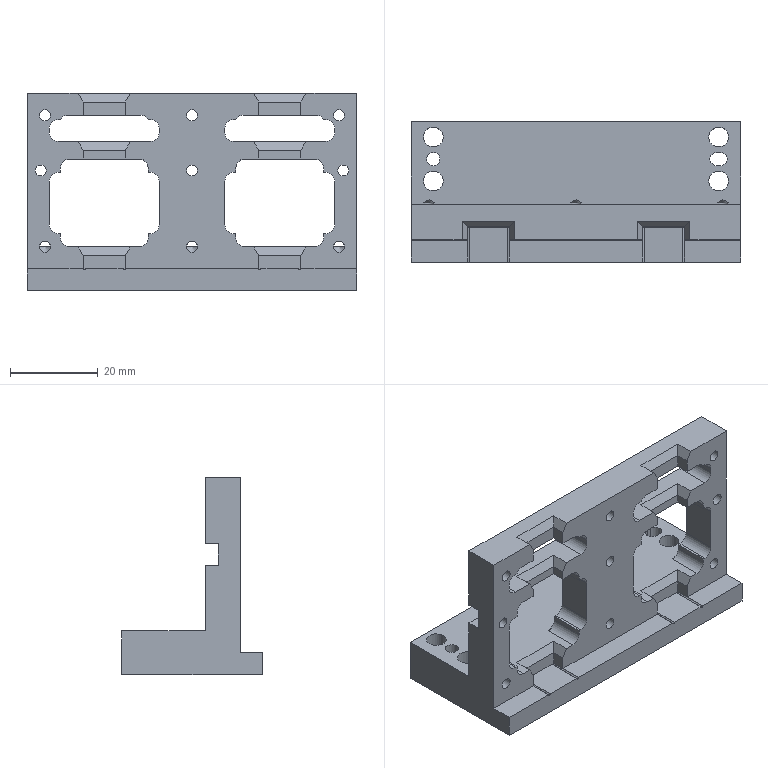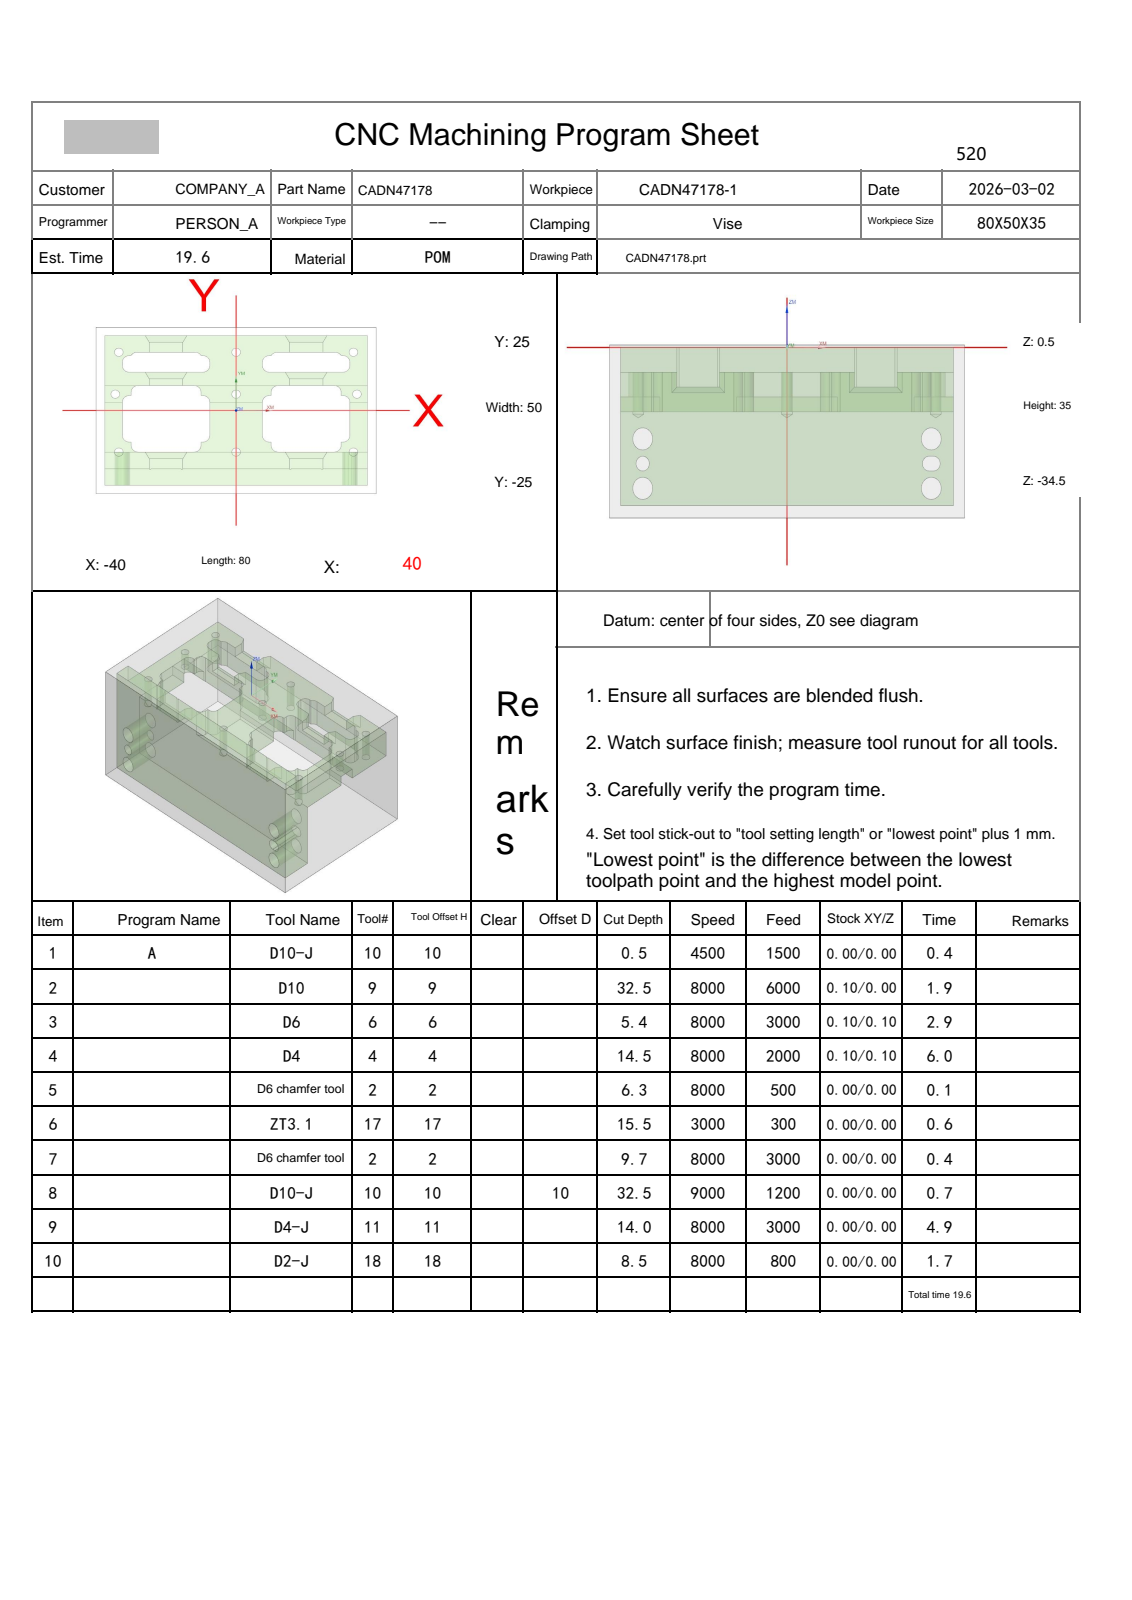NC program | NX | posted by the shop | part box 75 x 32 x 45 mm
Lines 1 to 1488 of 18359:
%
O0001
(Machine time: 21.50 MIN)
(===Total Tool:8===)
(T10=D10-J  D=10.  R=0.   D-  H10 Z=-32.  )
(T9=D10     D=10.  R=0.   D-  H09 Z=-32.  )
(T6=D6      D=6.   R=0.   D-  H06 Z=-4.9  )
(T4=D4      D=4.   R=0.   D-  H04 Z=-14.  )
(T2=D6 chamfer tool   D=6.   R=0.   D-  H02 Z=-9.2  )
(T17=ZT3.1  D=3.1  DR_a=118 D-  H17 Z=-15.  )
(T11=D4-J   D=4.   R=0.   D11 H11 Z=-13.52)
(T18=D2-J   D=2.   R=0.   D-  H18 Z=-8.   )
G80 G90 G17 G49 G40
G91 G28 Z0
M01
N1 T10 M06
(D10-J  D=10. R=0. H=10 ce=0.00 di=0.00)
G00 G90 G54 X47.5 Y-20.625 M03 S4500
G43 H10 Z30.
M08
Z2.
G01 Z0.0 F1500.
X42.5
X-42.5
Y-13.75
X42.5
Y-6.875
X-42.5
Y0.0
X42.5
Y6.875
X-42.5
Y13.75
X42.5
Y20.625
X-42.5
X-47.5
Z2.
G00 Z30.
G91 G28 Z0.0
M05
M09
G91 G28 Z0.0
M01
N2 T09 M06
(D10  D=10. R=0. H=09 ce=0.10 di=0.00)
G00 G90 G54 X0.0 Y-27.6 M03 S8000
G43 H09 Z30.
M08
Z.5
G01 X-37.5 Z.391 F6000.
G02 X-42.6 Y-22.5 Z.367 I0.0 J5.1
G01 Y22.5 Z.236
G02 X-37.5 Y27.6 Z.213 I5.1 J0.0
G01 X37.5 Z-.006
G02 X42.6 Y22.5 Z-.029 I0.0 J-5.1
G01 Y-22.5 Z-.16
G02 X37.5 Y-27.6 Z-.183 I-5.1 J0.0
G01 X-37.5 Z-.402
G02 X-42.6 Y-22.5 Z-.425 I0.0 J5.1
G01 Y22.5 Z-.556
G02 X-37.5 Y27.6 Z-.58 I5.1 J0.0
G01 X37.5 Z-.798
G02 X42.6 Y22.5 Z-.822 I0.0 J-5.1
G01 Y-22.5 Z-.953
G02 X37.5 Y-27.6 Z-.976 I-5.1 J0.0
G01 X-37.5 Z-1.195
G02 X-42.6 Y-22.5 Z-1.218 I0.0 J5.1
G01 Y22.5 Z-1.349
G02 X-37.5 Y27.6 Z-1.372 I5.1 J0.0
G01 X37.5 Z-1.591
G02 X42.6 Y22.5 Z-1.614 I0.0 J-5.1
G01 Y-22.5 Z-1.745
G02 X37.5 Y-27.6 Z-1.769 I-5.1 J0.0
G01 X-37.5 Z-1.987
G02 X-42.6 Y-22.5 Z-2.011 I0.0 J5.1
G01 Y22.5 Z-2.142
G02 X-37.5 Y27.6 Z-2.165 I5.1 J0.0
G01 X37.5 Z-2.384
G02 X42.6 Y22.5 Z-2.407 I0.0 J-5.1
G01 Y-22.5 Z-2.538
G02 X37.5 Y-27.6 Z-2.561 I-5.1 J0.0
G01 X-37.5 Z-2.78
G02 X-42.6 Y-22.5 Z-2.803 I0.0 J5.1
G01 Y22.5 Z-2.934
G02 X-37.5 Y27.6 Z-2.958 I5.1 J0.0
G01 X37.5 Z-3.176
G02 X42.6 Y22.5 Z-3.2 I0.0 J-5.1
G01 Y-22.5 Z-3.331
G02 X37.5 Y-27.6 Z-3.354 I-5.1 J0.0
G01 X-37.5 Z-3.573
G02 X-42.6 Y-22.5 Z-3.596 I0.0 J5.1
G01 Y22.5 Z-3.727
G02 X-37.5 Y27.6 Z-3.75 I5.1 J0.0
G01 X37.5 Z-3.969
G02 X42.6 Y22.5 Z-3.992 I0.0 J-5.1
G01 Y-22.5 Z-4.123
G02 X37.5 Y-27.6 Z-4.147 I-5.1 J0.0
G01 X-37.5 Z-4.365
G02 X-42.6 Y-22.5 Z-4.389 I0.0 J5.1
G01 Y22.5 Z-4.52
G02 X-37.5 Y27.6 Z-4.543 I5.1 J0.0
G01 X37.5 Z-4.762
G02 X42.6 Y22.5 Z-4.785 I0.0 J-5.1
G01 Y-22.5 Z-4.916
G02 X37.5 Y-27.6 Z-4.94 I-5.1 J0.0
G01 X-37.5 Z-5.158
G02 X-42.6 Y-22.5 Z-5.181 I0.0 J5.1
G01 Y22.5 Z-5.313
G02 X-37.5 Y27.6 Z-5.336 I5.1 J0.0
G01 X37.5 Z-5.554
G02 X42.6 Y22.5 Z-5.578 I0.0 J-5.1
G01 Y-22.5 Z-5.709
G02 X37.5 Y-27.6 Z-5.732 I-5.1 J0.0
G01 X-37.5 Z-5.951
G02 X-42.6 Y-22.5 Z-5.974 I0.0 J5.1
G01 Y22.5 Z-6.105
G02 X-37.5 Y27.6 Z-6.129 I5.1 J0.0
G01 X37.5 Z-6.347
G02 X42.6 Y22.5 Z-6.37 I0.0 J-5.1
G01 Y-22.5 Z-6.502
G02 X37.5 Y-27.6 Z-6.525 I-5.1 J0.0
G01 X-37.5 Z-6.743
G02 X-42.6 Y-22.5 Z-6.767 I0.0 J5.1
G01 Y22.5 Z-6.898
G02 X-37.5 Y27.6 Z-6.921 I5.1 J0.0
G01 X37.5 Z-7.14
G02 X42.6 Y22.5 Z-7.163 I0.0 J-5.1
G01 Y-22.5 Z-7.294
G02 X37.5 Y-27.6 Z-7.318 I-5.1 J0.0
G01 X-37.5 Z-7.536
G02 X-42.6 Y-22.5 Z-7.559 I0.0 J5.1
G01 Y22.5 Z-7.691
G02 X-37.5 Y27.6 Z-7.714 I5.1 J0.0
G01 X37.5 Z-7.932
G02 X42.6 Y22.5 Z-7.956 I0.0 J-5.1
G01 Y-22.5 Z-8.087
G02 X37.5 Y-27.6 Z-8.11 I-5.1 J0.0
G01 X-37.5 Z-8.329
G02 X-42.6 Y-22.5 Z-8.352 I0.0 J5.1
G01 Y22.5 Z-8.483
G02 X-37.5 Y27.6 Z-8.507 I5.1 J0.0
G01 X37.5 Z-8.725
G02 X42.6 Y22.5 Z-8.748 I0.0 J-5.1
G01 Y-22.5 Z-8.88
G02 X37.5 Y-27.6 Z-8.903 I-5.1 J0.0
G01 X-37.5 Z-9.121
G02 X-42.6 Y-22.5 Z-9.145 I0.0 J5.1
G01 Y22.5 Z-9.276
G02 X-37.5 Y27.6 Z-9.299 I5.1 J0.0
G01 X37.5 Z-9.518
G02 X42.6 Y22.5 Z-9.541 I0.0 J-5.1
G01 Y-22.5 Z-9.672
G02 X37.5 Y-27.6 Z-9.696 I-5.1 J0.0
G01 X-37.5 Z-9.914
G02 X-42.6 Y-22.5 Z-9.937 I0.0 J5.1
G01 Y22.5 Z-10.069
G02 X-37.5 Y27.6 Z-10.092 I5.1 J0.0
G01 X37.5 Z-10.31
G02 X42.6 Y22.5 Z-10.334 I0.0 J-5.1
G01 Y-22.5 Z-10.465
G02 X37.5 Y-27.6 Z-10.488 I-5.1 J0.0
G01 X-37.5 Z-10.707
G02 X-42.6 Y-22.5 Z-10.73 I0.0 J5.1
G01 Y22.5 Z-10.861
G02 X-37.5 Y27.6 Z-10.885 I5.1 J0.0
G01 X37.5 Z-11.103
G02 X42.6 Y22.5 Z-11.127 I0.0 J-5.1
G01 Y-22.5 Z-11.258
G02 X37.5 Y-27.6 Z-11.281 I-5.1 J0.0
G01 X-37.5 Z-11.5
G02 X-42.6 Y-22.5 Z-11.523 I0.0 J5.1
G01 Y22.5 Z-11.654
G02 X-37.5 Y27.6 Z-11.677 I5.1 J0.0
G01 X37.5 Z-11.896
G02 X42.6 Y22.5 Z-11.919 I0.0 J-5.1
G01 Y-22.5 Z-12.05
G02 X37.5 Y-27.6 Z-12.074 I-5.1 J0.0
G01 X-37.5 Z-12.292
G02 X-42.6 Y-22.5 Z-12.316 I0.0 J5.1
G01 Y22.5 Z-12.447
G02 X-37.5 Y27.6 Z-12.47 I5.1 J0.0
G01 X37.5 Z-12.689
G02 X42.6 Y22.5 Z-12.712 I0.0 J-5.1
G01 Y-22.5 Z-12.843
G02 X37.5 Y-27.6 Z-12.866 I-5.1 J0.0
G01 X-37.5 Z-13.085
G02 X-42.6 Y-22.5 Z-13.108 I0.0 J5.1
G01 Y22.5 Z-13.239
G02 X-37.5 Y27.6 Z-13.263 I5.1 J0.0
G01 X37.5 Z-13.481
G02 X42.6 Y22.5 Z-13.505 I0.0 J-5.1
G01 Y-22.5 Z-13.636
G02 X37.5 Y-27.6 Z-13.659 I-5.1 J0.0
G01 X-37.5 Z-13.878
G02 X-42.6 Y-22.5 Z-13.901 I0.0 J5.1
G01 Y22.5 Z-14.032
G02 X-37.5 Y27.6 Z-14.055 I5.1 J0.0
G01 X37.5 Z-14.274
G02 X42.6 Y22.5 Z-14.297 I0.0 J-5.1
G01 Y-22.5 Z-14.428
G02 X37.5 Y-27.6 Z-14.452 I-5.1 J0.0
G01 X-37.5 Z-14.67
G02 X-42.6 Y-22.5 Z-14.694 I0.0 J5.1
G01 Y22.5 Z-14.825
G02 X-37.5 Y27.6 Z-14.848 I5.1 J0.0
G01 X37.5 Z-15.067
G02 X42.6 Y22.5 Z-15.09 I0.0 J-5.1
G01 Y-22.5 Z-15.221
G02 X37.5 Y-27.6 Z-15.244 I-5.1 J0.0
G01 X-37.5 Z-15.463
G02 X-42.6 Y-22.5 Z-15.486 I0.0 J5.1
G01 Y22.5 Z-15.617
G02 X-37.5 Y27.6 Z-15.641 I5.1 J0.0
G01 X37.5 Z-15.859
G02 X42.6 Y22.5 Z-15.883 I0.0 J-5.1
G01 Y-22.5 Z-16.014
G02 X37.5 Y-27.6 Z-16.037 I-5.1 J0.0
G01 X-37.5 Z-16.256
G02 X-42.6 Y-22.5 Z-16.279 I0.0 J5.1
G01 Y22.5 Z-16.41
G02 X-37.5 Y27.6 Z-16.433 I5.1 J0.0
G01 X37.5 Z-16.652
G02 X42.6 Y22.5 Z-16.675 I0.0 J-5.1
G01 Y-22.5 Z-16.806
G02 X37.5 Y-27.6 Z-16.83 I-5.1 J0.0
G01 X-37.5 Z-17.048
G02 X-42.6 Y-22.5 Z-17.072 I0.0 J5.1
G01 Y22.5 Z-17.203
G02 X-37.5 Y27.6 Z-17.226 I5.1 J0.0
G01 X37.5 Z-17.445
G02 X42.6 Y22.5 Z-17.468 I0.0 J-5.1
G01 Y-22.5 Z-17.599
G02 X37.5 Y-27.6 Z-17.622 I-5.1 J0.0
G01 X-37.5 Z-17.841
G02 X-42.6 Y-22.5 Z-17.864 I0.0 J5.1
G01 Y22.5 Z-17.995
G02 X-37.5 Y27.6 Z-18.019 I5.1 J0.0
G01 X37.5 Z-18.237
G02 X42.6 Y22.5 Z-18.261 I0.0 J-5.1
G01 Y-22.5 Z-18.392
G02 X37.5 Y-27.6 Z-18.415 I-5.1 J0.0
G01 X-37.5 Z-18.634
G02 X-42.6 Y-22.5 Z-18.657 I0.0 J5.1
G01 Y22.5 Z-18.788
G02 X-37.5 Y27.6 Z-18.811 I5.1 J0.0
G01 X37.5 Z-19.03
G02 X42.6 Y22.5 Z-19.053 I0.0 J-5.1
G01 Y-22.5 Z-19.184
G02 X37.5 Y-27.6 Z-19.208 I-5.1 J0.0
G01 X-37.5 Z-19.426
G02 X-42.6 Y-22.5 Z-19.45 I0.0 J5.1
G01 Y22.5 Z-19.581
G02 X-37.5 Y27.6 Z-19.604 I5.1 J0.0
G01 X37.5 Z-19.823
G02 X42.6 Y22.5 Z-19.846 I0.0 J-5.1
G01 Y-22.5 Z-19.977
G02 X37.5 Y-27.6 Z-20. I-5.1 J0.0
G01 X-37.5 Z-20.219
G02 X-42.6 Y-22.5 Z-20.242 I0.0 J5.1
G01 Y22.5 Z-20.373
G02 X-37.5 Y27.6 Z-20.397 I5.1 J0.0
G01 X37.5 Z-20.615
G02 X42.6 Y22.5 Z-20.639 I0.0 J-5.1
G01 Y-22.5 Z-20.77
G02 X37.5 Y-27.6 Z-20.793 I-5.1 J0.0
G01 X-37.5 Z-21.012
G02 X-42.6 Y-22.5 Z-21.035 I0.0 J5.1
G01 Y22.5 Z-21.166
G02 X-37.5 Y27.6 Z-21.19 I5.1 J0.0
G01 X37.5 Z-21.408
G02 X42.6 Y22.5 Z-21.431 I0.0 J-5.1
G01 Y-22.5 Z-21.563
G02 X37.5 Y-27.6 Z-21.586 I-5.1 J0.0
G01 X-37.5 Z-21.804
G02 X-42.6 Y-22.5 Z-21.828 I0.0 J5.1
G01 Y22.5 Z-21.959
G02 X-37.5 Y27.6 Z-21.982 I5.1 J0.0
G01 X37.5 Z-22.201
G02 X42.6 Y22.5 Z-22.224 I0.0 J-5.1
G01 Y-22.5 Z-22.355
G02 X37.5 Y-27.6 Z-22.379 I-5.1 J0.0
G01 X-37.5 Z-22.597
G02 X-42.6 Y-22.5 Z-22.62 I0.0 J5.1
G01 Y22.5 Z-22.752
G02 X-37.5 Y27.6 Z-22.775 I5.1 J0.0
G01 X37.5 Z-22.993
G02 X42.6 Y22.5 Z-23.017 I0.0 J-5.1
G01 Y-22.5 Z-23.148
G02 X37.5 Y-27.6 Z-23.171 I-5.1 J0.0
G01 X-37.5 Z-23.39
G02 X-42.6 Y-22.5 Z-23.413 I0.0 J5.1
G01 Y22.5 Z-23.544
G02 X-37.5 Y27.6 Z-23.568 I5.1 J0.0
G01 X37.5 Z-23.786
G02 X42.6 Y22.5 Z-23.809 I0.0 J-5.1
G01 Y-22.5 Z-23.941
G02 X37.5 Y-27.6 Z-23.964 I-5.1 J0.0
G01 X-37.5 Z-24.182
G02 X-42.6 Y-22.5 Z-24.206 I0.0 J5.1
G01 Y22.5 Z-24.337
G02 X-37.5 Y27.6 Z-24.36 I5.1 J0.0
G01 X37.5 Z-24.579
G02 X42.6 Y22.5 Z-24.602 I0.0 J-5.1
G01 Y-22.5 Z-24.733
G02 X37.5 Y-27.6 Z-24.757 I-5.1 J0.0
G01 X-37.5 Z-24.975
G02 X-42.6 Y-22.5 Z-24.998 I0.0 J5.1
G01 Y22.5 Z-25.13
G02 X-37.5 Y27.6 Z-25.153 I5.1 J0.0
G01 X37.5 Z-25.371
G02 X42.6 Y22.5 Z-25.395 I0.0 J-5.1
G01 Y-22.5 Z-25.526
G02 X37.5 Y-27.6 Z-25.549 I-5.1 J0.0
G01 X-37.5 Z-25.768
G02 X-42.6 Y-22.5 Z-25.791 I0.0 J5.1
G01 Y22.5 Z-25.922
G02 X-37.5 Y27.6 Z-25.946 I5.1 J0.0
G01 X37.5 Z-26.164
G02 X42.6 Y22.5 Z-26.187 I0.0 J-5.1
G01 Y-22.5 Z-26.319
G02 X37.5 Y-27.6 Z-26.342 I-5.1 J0.0
G01 X-37.5 Z-26.56
G02 X-42.6 Y-22.5 Z-26.584 I0.0 J5.1
G01 Y22.5 Z-26.715
G02 X-37.5 Y27.6 Z-26.738 I5.1 J0.0
G01 X37.5 Z-26.957
G02 X42.6 Y22.5 Z-26.98 I0.0 J-5.1
G01 Y-22.5 Z-27.111
G02 X37.5 Y-27.6 Z-27.135 I-5.1 J0.0
G01 X-37.5 Z-27.353
G02 X-42.6 Y-22.5 Z-27.377 I0.0 J5.1
G01 Y22.5 Z-27.508
G02 X-37.5 Y27.6 Z-27.531 I5.1 J0.0
G01 X37.5 Z-27.75
G02 X42.6 Y22.5 Z-27.773 I0.0 J-5.1
G01 Y-22.5 Z-27.904
G02 X37.5 Y-27.6 Z-27.927 I-5.1 J0.0
G01 X-37.5 Z-28.146
G02 X-42.6 Y-22.5 Z-28.169 I0.0 J5.1
G01 Y22.5 Z-28.3
G02 X-37.5 Y27.6 Z-28.324 I5.1 J0.0
G01 X37.5 Z-28.542
G02 X42.6 Y22.5 Z-28.566 I0.0 J-5.1
G01 Y-22.5 Z-28.697
G02 X37.5 Y-27.6 Z-28.72 I-5.1 J0.0
G01 X-37.5 Z-28.939
G02 X-42.6 Y-22.5 Z-28.962 I0.0 J5.1
G01 Y22.5 Z-29.093
G02 X-37.5 Y27.6 Z-29.116 I5.1 J0.0
G01 X37.5 Z-29.335
G02 X42.6 Y22.5 Z-29.358 I0.0 J-5.1
G01 Y-22.5 Z-29.489
G02 X37.5 Y-27.6 Z-29.513 I-5.1 J0.0
G01 X-37.5 Z-29.731
G02 X-42.6 Y-22.5 Z-29.755 I0.0 J5.1
G01 Y22.5 Z-29.886
G02 X-37.5 Y27.6 Z-29.909 I5.1 J0.0
G01 X37.5 Z-30.128
G02 X42.6 Y22.5 Z-30.151 I0.0 J-5.1
G01 Y-22.5 Z-30.282
G02 X37.5 Y-27.6 Z-30.305 I-5.1 J0.0
G01 X-37.5 Z-30.524
G02 X-42.6 Y-22.5 Z-30.547 I0.0 J5.1
G01 Y22.5 Z-30.678
G02 X-37.5 Y27.6 Z-30.702 I5.1 J0.0
G01 X37.5 Z-30.92
G02 X42.6 Y22.5 Z-30.944 I0.0 J-5.1
G01 Y-22.5 Z-31.075
G02 X37.5 Y-27.6 Z-31.098 I-5.1 J0.0
G01 X-37.5 Z-31.317
G02 X-42.6 Y-22.5 Z-31.34 I0.0 J5.1
G01 Y22.5 Z-31.471
G02 X-37.5 Y27.6 Z-31.494 I5.1 J0.0
G01 X37.5 Z-31.713
G02 X42.6 Y22.5 Z-31.736 I0.0 J-5.1
G01 Y-22.5 Z-31.867
G02 X37.5 Y-27.6 Z-31.891 I-5.1 J0.0
G01 X0.0 Z-32.
X-37.5
G02 X-42.6 Y-22.5 I0.0 J5.1
G01 Y22.5
G02 X-37.5 Y27.6 I5.1 J0.0
G01 X37.5
G02 X42.6 Y22.5 I0.0 J-5.1
G01 Y-22.5
G02 X37.5 Y-27.6 I-5.1 J0.0
G01 X0.0
X-.5
Z-31.
G00 Z30.
G91 G28 Z0.0
M05
M09
G91 G28 Z0.0
M01
N3 T06 M06
(D6  D=6. R=0. H=06 ce=0.10 di=0.10)
G00 G90 G54 X0.0 Y28.5 M03 S8000
G43 H06 Z10.5
M08
Z1.01
G01 Z-.49 F3000.
Y25.44
X40.44
Y-14.4
X24.8
G03 X24.55 Y-14.41 I0.0 J-3.1
X24.3 Y-14.4 I-.25 J-3.09
G01 X15.7
G03 X15.45 Y-14.41 I0.0 J-3.1
X15.2 Y-14.4 I-.25 J-3.09
G01 X-15.2
G03 X-15.45 Y-14.41 I0.0 J-3.1
X-15.7 Y-14.4 I-.25 J-3.09
G01 X-24.3
G03 X-24.55 Y-14.41 I0.0 J-3.1
X-24.8 Y-14.4 I-.25 J-3.09
G01 X-40.44
Y25.44
X-1.821
G02 X-1.322 Y25.173 I0.0 J-.6
G01 X1.322 Y21.207
G03 X1.821 Y20.94 I.499 J.333
G01 X35.342
G02 X35.94 Y20.342 I-.002 J-.6
G01 Y-9.302
G02 X35.342 Y-9.9 I-.6 J.002
G01 X24.8
G03 X24.55 Y-9.904 I0.0 J-7.6
X24.3 Y-9.9 I-.25 J-7.596
G01 X15.7
G03 X15.45 Y-9.904 I0.0 J-7.6
X15.2 Y-9.9 I-.25 J-7.596
G01 X-15.2
G03 X-15.45 Y-9.904 I0.0 J-7.6
X-15.7 Y-9.9 I-.25 J-7.596
G01 X-24.3
G03 X-24.55 Y-9.904 I0.0 J-7.6
X-24.8 Y-9.9 I-.25 J-7.596
G01 X-35.342
G02 X-35.94 Y-9.302 I.002 J.6
G01 Y20.342
G02 X-35.342 Y20.94 I.6 J-.002
G01 X-1.821
G02 X-1.322 Y20.673 I0.0 J-.6
G01 X1.322 Y16.707
G03 X1.821 Y16.44 I.499 J.333
G01 X30.842
G02 X31.44 Y15.842 I-.002 J-.6
G01 Y-4.802
G02 X30.842 Y-5.4 I-.6 J.002
G01 X24.8
G03 X24.55 Y-5.403 I0.0 J-12.1
X24.3 Y-5.4 I-.25 J-12.097
G01 X15.7
G03 X15.45 Y-5.403 I0.0 J-12.1
X15.2 Y-5.4 I-.25 J-12.097
G01 X-15.2
G03 X-15.45 Y-5.403 I0.0 J-12.1
X-15.7 Y-5.4 I-.25 J-12.097
G01 X-24.3
G03 X-24.55 Y-5.403 I0.0 J-12.1
X-24.8 Y-5.4 I-.25 J-12.097
G01 X-30.842
G02 X-31.44 Y-4.802 I.002 J.6
G01 Y15.842
G02 X-30.842 Y16.44 I.6 J-.002
G01 X-1.821
G02 X-1.322 Y16.173 I0.0 J-.6
G01 X1.322 Y12.207
G03 X1.821 Y11.94 I.499 J.333
G01 X26.342
G02 X26.94 Y11.342 I-.002 J-.6
G01 Y-.302
G02 X26.342 Y-.9 I-.6 J.002
G01 X24.8
G03 X24.55 Y-.902 I0.0 J-16.6
X24.3 Y-.9 I-.25 J-16.598
G01 X15.7
G03 X15.45 Y-.902 I0.0 J-16.6
X15.2 Y-.9 I-.25 J-16.598
G01 X-15.2
G03 X-15.45 Y-.902 I0.0 J-16.6
X-15.7 Y-.9 I-.25 J-16.598
G01 X-24.3
G03 X-24.55 Y-.902 I0.0 J-16.6
X-24.8 Y-.9 I-.25 J-16.598
G01 X-26.342
G02 X-26.94 Y-.302 I.002 J.6
G01 Y11.342
G02 X-26.342 Y11.94 I.6 J-.002
G01 X-1.821
G02 X-1.322 Y11.673 I0.0 J-.6
G01 X1.322 Y7.707
G03 X1.821 Y7.44 I.499 J.333
G01 X21.842
G02 X22.44 Y6.842 I-.002 J-.6
G01 Y4.198
G02 X21.842 Y3.6 I-.6 J.002
G01 X-21.842
G02 X-22.44 Y4.198 I.002 J.6
G01 Y6.842
G02 X-21.842 Y7.44 I.6 J-.002
G01 X0.0
X.5
Y10.44
Z1.01
G00 X0.0 Y28.5
Z.52
G01 Z-.98
Y25.44
X40.44
Y-14.4
X24.8
G03 X24.55 Y-14.41 I0.0 J-3.1
X24.3 Y-14.4 I-.25 J-3.09
G01 X15.7
G03 X15.45 Y-14.41 I0.0 J-3.1
X15.2 Y-14.4 I-.25 J-3.09
G01 X-15.2
G03 X-15.45 Y-14.41 I0.0 J-3.1
X-15.7 Y-14.4 I-.25 J-3.09
G01 X-24.3
G03 X-24.55 Y-14.41 I0.0 J-3.1
X-24.8 Y-14.4 I-.25 J-3.09
G01 X-40.44
Y25.44
X-1.821
G02 X-1.322 Y25.173 I0.0 J-.6
G01 X1.322 Y21.207
G03 X1.821 Y20.94 I.499 J.333
G01 X35.342
G02 X35.94 Y20.342 I-.002 J-.6
G01 Y-9.302
G02 X35.342 Y-9.9 I-.6 J.002
G01 X24.8
G03 X24.55 Y-9.904 I0.0 J-7.6
X24.3 Y-9.9 I-.25 J-7.596
G01 X15.7
G03 X15.45 Y-9.904 I0.0 J-7.6
X15.2 Y-9.9 I-.25 J-7.596
G01 X-15.2
G03 X-15.45 Y-9.904 I0.0 J-7.6
X-15.7 Y-9.9 I-.25 J-7.596
G01 X-24.3
G03 X-24.55 Y-9.904 I0.0 J-7.6
X-24.8 Y-9.9 I-.25 J-7.596
G01 X-35.342
G02 X-35.94 Y-9.302 I.002 J.6
G01 Y20.342
G02 X-35.342 Y20.94 I.6 J-.002
G01 X-1.821
G02 X-1.322 Y20.673 I0.0 J-.6
G01 X1.322 Y16.707
G03 X1.821 Y16.44 I.499 J.333
G01 X30.842
G02 X31.44 Y15.842 I-.002 J-.6
G01 Y-4.802
G02 X30.842 Y-5.4 I-.6 J.002
G01 X24.8
G03 X24.55 Y-5.403 I0.0 J-12.1
X24.3 Y-5.4 I-.25 J-12.097
G01 X15.7
G03 X15.45 Y-5.403 I0.0 J-12.1
X15.2 Y-5.4 I-.25 J-12.097
G01 X-15.2
G03 X-15.45 Y-5.403 I0.0 J-12.1
X-15.7 Y-5.4 I-.25 J-12.097
G01 X-24.3
G03 X-24.55 Y-5.403 I0.0 J-12.1
X-24.8 Y-5.4 I-.25 J-12.097
G01 X-30.842
G02 X-31.44 Y-4.802 I.002 J.6
G01 Y15.842
G02 X-30.842 Y16.44 I.6 J-.002
G01 X-1.821
G02 X-1.322 Y16.173 I0.0 J-.6
G01 X1.322 Y12.207
G03 X1.821 Y11.94 I.499 J.333
G01 X26.342
G02 X26.94 Y11.342 I-.002 J-.6
G01 Y-.302
G02 X26.342 Y-.9 I-.6 J.002
G01 X24.8
G03 X24.55 Y-.902 I0.0 J-16.6
X24.3 Y-.9 I-.25 J-16.598
G01 X15.7
G03 X15.45 Y-.902 I0.0 J-16.6
X15.2 Y-.9 I-.25 J-16.598
G01 X-15.2
G03 X-15.45 Y-.902 I0.0 J-16.6
X-15.7 Y-.9 I-.25 J-16.598
G01 X-24.3
G03 X-24.55 Y-.902 I0.0 J-16.6
X-24.8 Y-.9 I-.25 J-16.598
G01 X-26.342
G02 X-26.94 Y-.302 I.002 J.6
G01 Y11.342
G02 X-26.342 Y11.94 I.6 J-.002
G01 X-1.821
G02 X-1.322 Y11.673 I0.0 J-.6
G01 X1.322 Y7.707
G03 X1.821 Y7.44 I.499 J.333
G01 X21.842
G02 X22.44 Y6.842 I-.002 J-.6
G01 Y4.198
G02 X21.842 Y3.6 I-.6 J.002
G01 X-21.842
G02 X-22.44 Y4.198 I.002 J.6
G01 Y6.842
G02 X-21.842 Y7.44 I.6 J-.002
G01 X0.0
X.5
Y10.44
Z.52
G00 X0.0 Y28.5
Z.03
G01 Z-1.47
Y25.44
X40.44
Y-14.4
X24.8
G03 X24.55 Y-14.41 I0.0 J-3.1
X24.3 Y-14.4 I-.25 J-3.09
G01 X15.7
G03 X15.45 Y-14.41 I0.0 J-3.1
X15.2 Y-14.4 I-.25 J-3.09
G01 X-15.2
G03 X-15.45 Y-14.41 I0.0 J-3.1
X-15.7 Y-14.4 I-.25 J-3.09
G01 X-24.3
G03 X-24.55 Y-14.41 I0.0 J-3.1
X-24.8 Y-14.4 I-.25 J-3.09
G01 X-40.44
Y25.44
X-1.821
G02 X-1.322 Y25.173 I0.0 J-.6
G01 X1.322 Y21.207
G03 X1.821 Y20.94 I.499 J.333
G01 X35.342
G02 X35.94 Y20.342 I-.002 J-.6
G01 Y-9.302
G02 X35.342 Y-9.9 I-.6 J.002
G01 X24.8
G03 X24.55 Y-9.904 I0.0 J-7.6
X24.3 Y-9.9 I-.25 J-7.596
G01 X15.7
G03 X15.45 Y-9.904 I0.0 J-7.6
X15.2 Y-9.9 I-.25 J-7.596
G01 X-15.2
G03 X-15.45 Y-9.904 I0.0 J-7.6
X-15.7 Y-9.9 I-.25 J-7.596
G01 X-24.3
G03 X-24.55 Y-9.904 I0.0 J-7.6
X-24.8 Y-9.9 I-.25 J-7.596
G01 X-35.342
G02 X-35.94 Y-9.302 I.002 J.6
G01 Y20.342
G02 X-35.342 Y20.94 I.6 J-.002
G01 X-1.821
G02 X-1.322 Y20.673 I0.0 J-.6
G01 X1.322 Y16.707
G03 X1.821 Y16.44 I.499 J.333
G01 X30.842
G02 X31.44 Y15.842 I-.002 J-.6
G01 Y-4.802
G02 X30.842 Y-5.4 I-.6 J.002
G01 X24.8
G03 X24.55 Y-5.403 I0.0 J-12.1
X24.3 Y-5.4 I-.25 J-12.097
G01 X15.7
G03 X15.45 Y-5.403 I0.0 J-12.1
X15.2 Y-5.4 I-.25 J-12.097
G01 X-15.2
G03 X-15.45 Y-5.403 I0.0 J-12.1
X-15.7 Y-5.4 I-.25 J-12.097
G01 X-24.3
G03 X-24.55 Y-5.403 I0.0 J-12.1
X-24.8 Y-5.4 I-.25 J-12.097
G01 X-30.842
G02 X-31.44 Y-4.802 I.002 J.6
G01 Y15.842
G02 X-30.842 Y16.44 I.6 J-.002
G01 X-1.821
G02 X-1.322 Y16.173 I0.0 J-.6
G01 X1.322 Y12.207
G03 X1.821 Y11.94 I.499 J.333
G01 X26.342
G02 X26.94 Y11.342 I-.002 J-.6
G01 Y-.302
G02 X26.342 Y-.9 I-.6 J.002
G01 X24.8
G03 X24.55 Y-.902 I0.0 J-16.6
X24.3 Y-.9 I-.25 J-16.598
G01 X15.7
G03 X15.45 Y-.902 I0.0 J-16.6
X15.2 Y-.9 I-.25 J-16.598
G01 X-15.2
G03 X-15.45 Y-.902 I0.0 J-16.6
X-15.7 Y-.9 I-.25 J-16.598
G01 X-24.3
G03 X-24.55 Y-.902 I0.0 J-16.6
X-24.8 Y-.9 I-.25 J-16.598
G01 X-26.342
G02 X-26.94 Y-.302 I.002 J.6
G01 Y11.342
G02 X-26.342 Y11.94 I.6 J-.002
G01 X-1.821
G02 X-1.322 Y11.673 I0.0 J-.6
G01 X1.322 Y7.707
G03 X1.821 Y7.44 I.499 J.333
G01 X21.842
G02 X22.44 Y6.842 I-.002 J-.6
G01 Y4.198
G02 X21.842 Y3.6 I-.6 J.002
G01 X-21.842
G02 X-22.44 Y4.198 I.002 J.6
G01 Y6.842
G02 X-21.842 Y7.44 I.6 J-.002
G01 X0.0
X.5
Y10.44
Z.03
G00 X0.0 Y28.5
Z-.46
G01 Z-1.96
Y25.44
X40.44
Y-14.4
X24.8
G03 X24.55 Y-14.41 I0.0 J-3.1
X24.3 Y-14.4 I-.25 J-3.09
G01 X15.7
G03 X15.45 Y-14.41 I0.0 J-3.1
X15.2 Y-14.4 I-.25 J-3.09
G01 X-15.2
G03 X-15.45 Y-14.41 I0.0 J-3.1
X-15.7 Y-14.4 I-.25 J-3.09
G01 X-24.3
G03 X-24.55 Y-14.41 I0.0 J-3.1
X-24.8 Y-14.4 I-.25 J-3.09
G01 X-40.44
Y25.44
X-1.821
G02 X-1.322 Y25.173 I0.0 J-.6
G01 X1.322 Y21.207
G03 X1.821 Y20.94 I.499 J.333
G01 X35.342
G02 X35.94 Y20.342 I-.002 J-.6
G01 Y-9.302
G02 X35.342 Y-9.9 I-.6 J.002
G01 X24.8
G03 X24.55 Y-9.904 I0.0 J-7.6
X24.3 Y-9.9 I-.25 J-7.596
G01 X15.7
G03 X15.45 Y-9.904 I0.0 J-7.6
X15.2 Y-9.9 I-.25 J-7.596
G01 X-15.2
G03 X-15.45 Y-9.904 I0.0 J-7.6
X-15.7 Y-9.9 I-.25 J-7.596
G01 X-24.3
G03 X-24.55 Y-9.904 I0.0 J-7.6
X-24.8 Y-9.9 I-.25 J-7.596
G01 X-35.342
G02 X-35.94 Y-9.302 I.002 J.6
G01 Y20.342
G02 X-35.342 Y20.94 I.6 J-.002
G01 X-1.821
G02 X-1.322 Y20.673 I0.0 J-.6
G01 X1.322 Y16.707
G03 X1.821 Y16.44 I.499 J.333
G01 X30.842
G02 X31.44 Y15.842 I-.002 J-.6
G01 Y-4.802
G02 X30.842 Y-5.4 I-.6 J.002
G01 X24.8
G03 X24.55 Y-5.403 I0.0 J-12.1
X24.3 Y-5.4 I-.25 J-12.097
G01 X15.7
G03 X15.45 Y-5.403 I0.0 J-12.1
X15.2 Y-5.4 I-.25 J-12.097
G01 X-15.2
G03 X-15.45 Y-5.403 I0.0 J-12.1
X-15.7 Y-5.4 I-.25 J-12.097
G01 X-24.3
G03 X-24.55 Y-5.403 I0.0 J-12.1
X-24.8 Y-5.4 I-.25 J-12.097
G01 X-30.842
G02 X-31.44 Y-4.802 I.002 J.6
G01 Y15.842
G02 X-30.842 Y16.44 I.6 J-.002
G01 X-1.821
G02 X-1.322 Y16.173 I0.0 J-.6
G01 X1.322 Y12.207
G03 X1.821 Y11.94 I.499 J.333
G01 X26.342
G02 X26.94 Y11.342 I-.002 J-.6
G01 Y-.302
G02 X26.342 Y-.9 I-.6 J.002
G01 X24.8
G03 X24.55 Y-.902 I0.0 J-16.6
X24.3 Y-.9 I-.25 J-16.598
G01 X15.7
G03 X15.45 Y-.902 I0.0 J-16.6
X15.2 Y-.9 I-.25 J-16.598
G01 X-15.2
G03 X-15.45 Y-.902 I0.0 J-16.6
X-15.7 Y-.9 I-.25 J-16.598
G01 X-24.3
G03 X-24.55 Y-.902 I0.0 J-16.6
X-24.8 Y-.9 I-.25 J-16.598
G01 X-26.342
G02 X-26.94 Y-.302 I.002 J.6
G01 Y11.342
G02 X-26.342 Y11.94 I.6 J-.002
G01 X-1.821
G02 X-1.322 Y11.673 I0.0 J-.6
G01 X1.322 Y7.707
G03 X1.821 Y7.44 I.499 J.333
G01 X21.842
G02 X22.44 Y6.842 I-.002 J-.6
G01 Y4.198
G02 X21.842 Y3.6 I-.6 J.002
G01 X-21.842
G02 X-22.44 Y4.198 I.002 J.6
G01 Y6.842
G02 X-21.842 Y7.44 I.6 J-.002
G01 X0.0
X.5
Y10.44
Z-.46
G00 X0.0 Y28.5
Z-.95
G01 Z-2.45
Y25.44
X40.44
Y-14.4
X24.8
G03 X24.55 Y-14.41 I0.0 J-3.1
X24.3 Y-14.4 I-.25 J-3.09
G01 X15.7
G03 X15.45 Y-14.41 I0.0 J-3.1
X15.2 Y-14.4 I-.25 J-3.09
G01 X-15.2
G03 X-15.45 Y-14.41 I0.0 J-3.1
X-15.7 Y-14.4 I-.25 J-3.09
G01 X-24.3
G03 X-24.55 Y-14.41 I0.0 J-3.1
X-24.8 Y-14.4 I-.25 J-3.09
G01 X-40.44
Y25.44
X-1.821
G02 X-1.322 Y25.173 I0.0 J-.6
G01 X1.322 Y21.207
G03 X1.821 Y20.94 I.499 J.333
G01 X35.342
G02 X35.94 Y20.342 I-.002 J-.6
G01 Y-9.302
G02 X35.342 Y-9.9 I-.6 J.002
G01 X24.8
G03 X24.55 Y-9.904 I0.0 J-7.6
X24.3 Y-9.9 I-.25 J-7.596
G01 X15.7
G03 X15.45 Y-9.904 I0.0 J-7.6
X15.2 Y-9.9 I-.25 J-7.596
G01 X-15.2
G03 X-15.45 Y-9.904 I0.0 J-7.6
X-15.7 Y-9.9 I-.25 J-7.596
G01 X-24.3
G03 X-24.55 Y-9.904 I0.0 J-7.6
X-24.8 Y-9.9 I-.25 J-7.596
G01 X-35.342
G02 X-35.94 Y-9.302 I.002 J.6
G01 Y20.342
G02 X-35.342 Y20.94 I.6 J-.002
G01 X-1.821
G02 X-1.322 Y20.673 I0.0 J-.6
G01 X1.322 Y16.707
G03 X1.821 Y16.44 I.499 J.333
G01 X30.842
G02 X31.44 Y15.842 I-.002 J-.6
G01 Y-4.802
G02 X30.842 Y-5.4 I-.6 J.002
G01 X24.8
G03 X24.55 Y-5.403 I0.0 J-12.1
X24.3 Y-5.4 I-.25 J-12.097
G01 X15.7
G03 X15.45 Y-5.403 I0.0 J-12.1
X15.2 Y-5.4 I-.25 J-12.097
G01 X-15.2
G03 X-15.45 Y-5.403 I0.0 J-12.1
X-15.7 Y-5.4 I-.25 J-12.097
G01 X-24.3
G03 X-24.55 Y-5.403 I0.0 J-12.1
X-24.8 Y-5.4 I-.25 J-12.097
G01 X-30.842
G02 X-31.44 Y-4.802 I.002 J.6
G01 Y15.842
G02 X-30.842 Y16.44 I.6 J-.002
G01 X-1.821
G02 X-1.322 Y16.173 I0.0 J-.6
G01 X1.322 Y12.207
G03 X1.821 Y11.94 I.499 J.333
G01 X26.342
G02 X26.94 Y11.342 I-.002 J-.6
G01 Y-.302
G02 X26.342 Y-.9 I-.6 J.002
G01 X24.8
G03 X24.55 Y-.902 I0.0 J-16.6
X24.3 Y-.9 I-.25 J-16.598
G01 X15.7
G03 X15.45 Y-.902 I0.0 J-16.6
X15.2 Y-.9 I-.25 J-16.598
G01 X-15.2
G03 X-15.45 Y-.902 I0.0 J-16.6
X-15.7 Y-.9 I-.25 J-16.598
G01 X-24.3
G03 X-24.55 Y-.902 I0.0 J-16.6
X-24.8 Y-.9 I-.25 J-16.598
G01 X-26.342
G02 X-26.94 Y-.302 I.002 J.6
G01 Y11.342
G02 X-26.342 Y11.94 I.6 J-.002
G01 X-1.821
G02 X-1.322 Y11.673 I0.0 J-.6
G01 X1.322 Y7.707
G03 X1.821 Y7.44 I.499 J.333
G01 X21.842
G02 X22.44 Y6.842 I-.002 J-.6
G01 Y4.198
G02 X21.842 Y3.6 I-.6 J.002
G01 X-21.842
G02 X-22.44 Y4.198 I.002 J.6
G01 Y6.842
G02 X-21.842 Y7.44 I.6 J-.002
G01 X0.0
X.5
Y10.44
Z-.95
G00 X0.0 Y28.5
Z-1.44
G01 Z-2.94
Y25.44
X40.44
Y-14.4
X24.8
G03 X24.55 Y-14.41 I0.0 J-3.1
X24.3 Y-14.4 I-.25 J-3.09
G01 X15.7
G03 X15.45 Y-14.41 I0.0 J-3.1
X15.2 Y-14.4 I-.25 J-3.09
G01 X-15.2
G03 X-15.45 Y-14.41 I0.0 J-3.1
X-15.7 Y-14.4 I-.25 J-3.09
G01 X-24.3
G03 X-24.55 Y-14.41 I0.0 J-3.1
X-24.8 Y-14.4 I-.25 J-3.09
G01 X-40.44
Y25.44
X-1.821
G02 X-1.322 Y25.173 I0.0 J-.6
G01 X1.322 Y21.207
G03 X1.821 Y20.94 I.499 J.333
G01 X35.342
G02 X35.94 Y20.342 I-.002 J-.6
G01 Y-9.302
G02 X35.342 Y-9.9 I-.6 J.002
G01 X24.8
G03 X24.55 Y-9.904 I0.0 J-7.6
X24.3 Y-9.9 I-.25 J-7.596
G01 X15.7
G03 X15.45 Y-9.904 I0.0 J-7.6
X15.2 Y-9.9 I-.25 J-7.596
G01 X-15.2
G03 X-15.45 Y-9.904 I0.0 J-7.6
X-15.7 Y-9.9 I-.25 J-7.596
G01 X-24.3
G03 X-24.55 Y-9.904 I0.0 J-7.6
X-24.8 Y-9.9 I-.25 J-7.596
G01 X-35.342
G02 X-35.94 Y-9.302 I.002 J.6
G01 Y20.342
G02 X-35.342 Y20.94 I.6 J-.002
G01 X-1.821
G02 X-1.322 Y20.673 I0.0 J-.6
G01 X1.322 Y16.707
G03 X1.821 Y16.44 I.499 J.333
G01 X30.842
G02 X31.44 Y15.842 I-.002 J-.6
G01 Y-4.802
G02 X30.842 Y-5.4 I-.6 J.002
G01 X24.8
G03 X24.55 Y-5.403 I0.0 J-12.1
X24.3 Y-5.4 I-.25 J-12.097
G01 X15.7
G03 X15.45 Y-5.403 I0.0 J-12.1
X15.2 Y-5.4 I-.25 J-12.097
G01 X-15.2
G03 X-15.45 Y-5.403 I0.0 J-12.1
X-15.7 Y-5.4 I-.25 J-12.097
G01 X-24.3
G03 X-24.55 Y-5.403 I0.0 J-12.1
X-24.8 Y-5.4 I-.25 J-12.097
G01 X-30.842
G02 X-31.44 Y-4.802 I.002 J.6
G01 Y15.842
G02 X-30.842 Y16.44 I.6 J-.002
G01 X-1.821
G02 X-1.322 Y16.173 I0.0 J-.6
G01 X1.322 Y12.207
G03 X1.821 Y11.94 I.499 J.333
G01 X26.342
G02 X26.94 Y11.342 I-.002 J-.6
G01 Y-.302
G02 X26.342 Y-.9 I-.6 J.002
G01 X24.8
G03 X24.55 Y-.902 I0.0 J-16.6
X24.3 Y-.9 I-.25 J-16.598
G01 X15.7
G03 X15.45 Y-.902 I0.0 J-16.6
X15.2 Y-.9 I-.25 J-16.598
G01 X-15.2
G03 X-15.45 Y-.902 I0.0 J-16.6
X-15.7 Y-.9 I-.25 J-16.598
G01 X-24.3
G03 X-24.55 Y-.902 I0.0 J-16.6
X-24.8 Y-.9 I-.25 J-16.598
G01 X-26.342
G02 X-26.94 Y-.302 I.002 J.6
G01 Y11.342
G02 X-26.342 Y11.94 I.6 J-.002
G01 X-1.821
G02 X-1.322 Y11.673 I0.0 J-.6
G01 X1.322 Y7.707
G03 X1.821 Y7.44 I.499 J.333
G01 X21.842
G02 X22.44 Y6.842 I-.002 J-.6
G01 Y4.198
G02 X21.842 Y3.6 I-.6 J.002
G01 X-21.842
G02 X-22.44 Y4.198 I.002 J.6
G01 Y6.842
G02 X-21.842 Y7.44 I.6 J-.002
G01 X0.0
X.5
Y10.44
Z-1.44
G00 X0.0 Y28.5
Z-1.93
G01 Z-3.43
Y25.44
X40.44
Y-14.4
X24.8
G03 X24.55 Y-14.41 I0.0 J-3.1
X24.3 Y-14.4 I-.25 J-3.09
G01 X15.7
G03 X15.45 Y-14.41 I0.0 J-3.1
X15.2 Y-14.4 I-.25 J-3.09
G01 X-15.2
G03 X-15.45 Y-14.41 I0.0 J-3.1
X-15.7 Y-14.4 I-.25 J-3.09
G01 X-24.3
G03 X-24.55 Y-14.41 I0.0 J-3.1
X-24.8 Y-14.4 I-.25 J-3.09
G01 X-40.44
Y25.44
X-1.821
G02 X-1.322 Y25.173 I0.0 J-.6
G01 X1.322 Y21.207
G03 X1.821 Y20.94 I.499 J.333
G01 X35.342
G02 X35.94 Y20.342 I-.002 J-.6
G01 Y-9.302
G02 X35.342 Y-9.9 I-.6 J.002
G01 X24.8
G03 X24.55 Y-9.904 I0.0 J-7.6
X24.3 Y-9.9 I-.25 J-7.596
G01 X15.7
G03 X15.45 Y-9.904 I0.0 J-7.6
X15.2 Y-9.9 I-.25 J-7.596
G01 X-15.2
G03 X-15.45 Y-9.904 I0.0 J-7.6
X-15.7 Y-9.9 I-.25 J-7.596
G01 X-24.3
G03 X-24.55 Y-9.904 I0.0 J-7.6
X-24.8 Y-9.9 I-.25 J-7.596
G01 X-35.342
G02 X-35.94 Y-9.302 I.002 J.6
G01 Y20.342
G02 X-35.342 Y20.94 I.6 J-.002
G01 X-1.821
G02 X-1.322 Y20.673 I0.0 J-.6
G01 X1.322 Y16.707
G03 X1.821 Y16.44 I.499 J.333
G01 X30.842
G02 X31.44 Y15.842 I-.002 J-.6
G01 Y-4.802
G02 X30.842 Y-5.4 I-.6 J.002
G01 X24.8
G03 X24.55 Y-5.403 I0.0 J-12.1
X24.3 Y-5.4 I-.25 J-12.097
G01 X15.7
G03 X15.45 Y-5.403 I0.0 J-12.1
X15.2 Y-5.4 I-.25 J-12.097
G01 X-15.2
G03 X-15.45 Y-5.403 I0.0 J-12.1
X-15.7 Y-5.4 I-.25 J-12.097
G01 X-24.3
G03 X-24.55 Y-5.403 I0.0 J-12.1
X-24.8 Y-5.4 I-.25 J-12.097
G01 X-30.842
G02 X-31.44 Y-4.802 I.002 J.6
G01 Y15.842
G02 X-30.842 Y16.44 I.6 J-.002
G01 X-1.821
G02 X-1.322 Y16.173 I0.0 J-.6
G01 X1.322 Y12.207
G03 X1.821 Y11.94 I.499 J.333
G01 X26.342
G02 X26.94 Y11.342 I-.002 J-.6
G01 Y-.302
G02 X26.342 Y-.9 I-.6 J.002
G01 X24.8
G03 X24.55 Y-.902 I0.0 J-16.6
X24.3 Y-.9 I-.25 J-16.598
G01 X15.7
G03 X15.45 Y-.902 I0.0 J-16.6
X15.2 Y-.9 I-.25 J-16.598
G01 X-15.2
G03 X-15.45 Y-.902 I0.0 J-16.6
X-15.7 Y-.9 I-.25 J-16.598
G01 X-24.3
G03 X-24.55 Y-.902 I0.0 J-16.6
X-24.8 Y-.9 I-.25 J-16.598
G01 X-26.342
G02 X-26.94 Y-.302 I.002 J.6
G01 Y11.342
G02 X-26.342 Y11.94 I.6 J-.002
G01 X-1.821
G02 X-1.322 Y11.673 I0.0 J-.6
G01 X1.322 Y7.707
G03 X1.821 Y7.44 I.499 J.333
G01 X21.842
G02 X22.44 Y6.842 I-.002 J-.6
G01 Y4.198
G02 X21.842 Y3.6 I-.6 J.002
G01 X-21.842
G02 X-22.44 Y4.198 I.002 J.6
G01 Y6.842
G02 X-21.842 Y7.44 I.6 J-.002
G01 X0.0
X.5
Y10.44
Z-1.93
G00 X0.0 Y28.5
Z-2.42
G01 Z-3.92
Y25.44
X40.44
Y-14.4
X24.8
G03 X24.55 Y-14.41 I0.0 J-3.1
X24.3 Y-14.4 I-.25 J-3.09
G01 X15.7
G03 X15.45 Y-14.41 I0.0 J-3.1
X15.2 Y-14.4 I-.25 J-3.09
G01 X-15.2
G03 X-15.45 Y-14.41 I0.0 J-3.1
X-15.7 Y-14.4 I-.25 J-3.09
G01 X-24.3
G03 X-24.55 Y-14.41 I0.0 J-3.1
X-24.8 Y-14.4 I-.25 J-3.09
G01 X-40.44
Y25.44
X-1.821
G02 X-1.322 Y25.173 I0.0 J-.6
G01 X1.322 Y21.207
G03 X1.821 Y20.94 I.499 J.333
G01 X35.342
G02 X35.94 Y20.342 I-.002 J-.6
G01 Y-9.302
G02 X35.342 Y-9.9 I-.6 J.002
G01 X24.8
G03 X24.55 Y-9.904 I0.0 J-7.6
X24.3 Y-9.9 I-.25 J-7.596
G01 X15.7
G03 X15.45 Y-9.904 I0.0 J-7.6
X15.2 Y-9.9 I-.25 J-7.596
G01 X-15.2
G03 X-15.45 Y-9.904 I0.0 J-7.6
X-15.7 Y-9.9 I-.25 J-7.596
G01 X-24.3
G03 X-24.55 Y-9.904 I0.0 J-7.6
X-24.8 Y-9.9 I-.25 J-7.596
G01 X-35.342
G02 X-35.94 Y-9.302 I.002 J.6
G01 Y20.342
G02 X-35.342 Y20.94 I.6 J-.002
G01 X-1.821
G02 X-1.322 Y20.673 I0.0 J-.6
G01 X1.322 Y16.707
G03 X1.821 Y16.44 I.499 J.333
G01 X30.842
G02 X31.44 Y15.842 I-.002 J-.6
G01 Y-4.802
G02 X30.842 Y-5.4 I-.6 J.002
G01 X24.8
G03 X24.55 Y-5.403 I0.0 J-12.1
X24.3 Y-5.4 I-.25 J-12.097
G01 X15.7
G03 X15.45 Y-5.403 I0.0 J-12.1
X15.2 Y-5.4 I-.25 J-12.097
G01 X-15.2
G03 X-15.45 Y-5.403 I0.0 J-12.1
X-15.7 Y-5.4 I-.25 J-12.097
G01 X-24.3
G03 X-24.55 Y-5.403 I0.0 J-12.1
X-24.8 Y-5.4 I-.25 J-12.097
G01 X-30.842
G02 X-31.44 Y-4.802 I.002 J.6
G01 Y15.842
G02 X-30.842 Y16.44 I.6 J-.002
G01 X-1.821
G02 X-1.322 Y16.173 I0.0 J-.6
G01 X1.322 Y12.207
G03 X1.821 Y11.94 I.499 J.333
G01 X26.342
G02 X26.94 Y11.342 I-.002 J-.6
G01 Y-.302
G02 X26.342 Y-.9 I-.6 J.002
G01 X24.8
G03 X24.55 Y-.902 I0.0 J-16.6
X24.3 Y-.9 I-.25 J-16.598
G01 X15.7
G03 X15.45 Y-.902 I0.0 J-16.6
X15.2 Y-.9 I-.25 J-16.598
G01 X-15.2
G03 X-15.45 Y-.902 I0.0 J-16.6
X-15.7 Y-.9 I-.25 J-16.598
G01 X-24.3
G03 X-24.55 Y-.902 I0.0 J-16.6
X-24.8 Y-.9 I-.25 J-16.598
G01 X-26.342
G02 X-26.94 Y-.302 I.002 J.6
G01 Y11.342
G02 X-26.342 Y11.94 I.6 J-.002
G01 X-1.821
G02 X-1.322 Y11.673 I0.0 J-.6
G01 X1.322 Y7.707
G03 X1.821 Y7.44 I.499 J.333
G01 X21.842
G02 X22.44 Y6.842 I-.002 J-.6
G01 Y4.198
G02 X21.842 Y3.6 I-.6 J.002
G01 X-21.842
G02 X-22.44 Y4.198 I.002 J.6
G01 Y6.842
G02 X-21.842 Y7.44 I.6 J-.002
G01 X0.0
X.5
Y10.44
Z-2.42
G00 X0.0 Y28.5
Z-2.91
G01 Z-4.41
Y25.44
X40.44
Y-14.4
X24.8
G03 X24.55 Y-14.41 I0.0 J-3.1
X24.3 Y-14.4 I-.25 J-3.09
G01 X15.7
G03 X15.45 Y-14.41 I0.0 J-3.1
X15.2 Y-14.4 I-.25 J-3.09
G01 X-15.2
G03 X-15.45 Y-14.41 I0.0 J-3.1
X-15.7 Y-14.4 I-.25 J-3.09
G01 X-24.3
G03 X-24.55 Y-14.41 I0.0 J-3.1
X-24.8 Y-14.4 I-.25 J-3.09
G01 X-40.44
Y25.44
X-1.821
G02 X-1.322 Y25.173 I0.0 J-.6
G01 X1.322 Y21.207
G03 X1.821 Y20.94 I.499 J.333
G01 X35.342
G02 X35.94 Y20.342 I-.002 J-.6
G01 Y-9.302
G02 X35.342 Y-9.9 I-.6 J.002
G01 X24.8
G03 X24.55 Y-9.904 I0.0 J-7.6
X24.3 Y-9.9 I-.25 J-7.596
G01 X15.7
G03 X15.45 Y-9.904 I0.0 J-7.6
X15.2 Y-9.9 I-.25 J-7.596
G01 X-15.2
G03 X-15.45 Y-9.904 I0.0 J-7.6
X-15.7 Y-9.9 I-.25 J-7.596
G01 X-24.3
G03 X-24.55 Y-9.904 I0.0 J-7.6
X-24.8 Y-9.9 I-.25 J-7.596
G01 X-35.342
G02 X-35.94 Y-9.302 I.002 J.6
G01 Y20.342
G02 X-35.342 Y20.94 I.6 J-.002
G01 X-1.821
G02 X-1.322 Y20.673 I0.0 J-.6
G01 X1.322 Y16.707
G03 X1.821 Y16.44 I.499 J.333
G01 X30.842
G02 X31.44 Y15.842 I-.002 J-.6
G01 Y-4.802
G02 X30.842 Y-5.4 I-.6 J.002
G01 X24.8
G03 X24.55 Y-5.403 I0.0 J-12.1
X24.3 Y-5.4 I-.25 J-12.097
G01 X15.7
G03 X15.45 Y-5.403 I0.0 J-12.1
X15.2 Y-5.4 I-.25 J-12.097
G01 X-15.2
G03 X-15.45 Y-5.403 I0.0 J-12.1
X-15.7 Y-5.4 I-.25 J-12.097
G01 X-24.3
G03 X-24.55 Y-5.403 I0.0 J-12.1
X-24.8 Y-5.4 I-.25 J-12.097
G01 X-30.842
G02 X-31.44 Y-4.802 I.002 J.6
G01 Y15.842
G02 X-30.842 Y16.44 I.6 J-.002
G01 X-1.821
G02 X-1.322 Y16.173 I0.0 J-.6
G01 X1.322 Y12.207
G03 X1.821 Y11.94 I.499 J.333
G01 X26.342
G02 X26.94 Y11.342 I-.002 J-.6
G01 Y-.302
G02 X26.342 Y-.9 I-.6 J.002
G01 X24.8
G03 X24.55 Y-.902 I0.0 J-16.6
X24.3 Y-.9 I-.25 J-16.598
G01 X15.7
G03 X15.45 Y-.902 I0.0 J-16.6
X15.2 Y-.9 I-.25 J-16.598
G01 X-15.2
G03 X-15.45 Y-.902 I0.0 J-16.6
X-15.7 Y-.9 I-.25 J-16.598
G01 X-24.3
G03 X-24.55 Y-.902 I0.0 J-16.6
X-24.8 Y-.9 I-.25 J-16.598
G01 X-26.342
G02 X-26.94 Y-.302 I.002 J.6
G01 Y11.342
G02 X-26.342 Y11.94 I.6 J-.002
G01 X-1.821
G02 X-1.322 Y11.673 I0.0 J-.6
G01 X1.322 Y7.707
G03 X1.821 Y7.44 I.499 J.333
G01 X21.842
G02 X22.44 Y6.842 I-.002 J-.6
G01 Y4.198
G02 X21.842 Y3.6 I-.6 J.002
G01 X-21.842
G02 X-22.44 Y4.198 I.002 J.6
G01 Y6.842
G02 X-21.842 Y7.44 I.6 J-.002
G01 X0.0
X.5
Y10.44
Z-2.91
G00 X0.0 Y28.5
Z-3.4
G01 Z-4.9
Y25.44
X40.44
Y-14.4
X24.8
G03 X24.55 Y-14.41 I0.0 J-3.1
X24.3 Y-14.4 I-.25 J-3.09
G01 X15.7
G03 X15.45 Y-14.41 I0.0 J-3.1
X15.2 Y-14.4 I-.25 J-3.09
G01 X-15.2
G03 X-15.45 Y-14.41 I0.0 J-3.1
X-15.7 Y-14.4 I-.25 J-3.09
G01 X-24.3
G03 X-24.55 Y-14.41 I0.0 J-3.1
X-24.8 Y-14.4 I-.25 J-3.09
G01 X-40.44
Y25.44
X-1.821
G02 X-1.322 Y25.173 I0.0 J-.6
G01 X1.322 Y21.207
G03 X1.821 Y20.94 I.499 J.333
G01 X35.342
G02 X35.94 Y20.342 I-.002 J-.6
G01 Y-9.302
G02 X35.342 Y-9.9 I-.6 J.002
G01 X24.8
G03 X24.55 Y-9.904 I0.0 J-7.6
X24.3 Y-9.9 I-.25 J-7.596
G01 X15.7
G03 X15.45 Y-9.904 I0.0 J-7.6
X15.2 Y-9.9 I-.25 J-7.596
G01 X-15.2
G03 X-15.45 Y-9.904 I0.0 J-7.6
X-15.7 Y-9.9 I-.25 J-7.596
G01 X-24.3
G03 X-24.55 Y-9.904 I0.0 J-7.6
X-24.8 Y-9.9 I-.25 J-7.596
G01 X-35.342
G02 X-35.94 Y-9.302 I.002 J.6
G01 Y20.342
G02 X-35.342 Y20.94 I.6 J-.002
G01 X-1.821
G02 X-1.322 Y20.673 I0.0 J-.6
G01 X1.322 Y16.707
G03 X1.821 Y16.44 I.499 J.333
G01 X30.842
G02 X31.44 Y15.842 I-.002 J-.6
G01 Y-4.802
G02 X30.842 Y-5.4 I-.6 J.002
G01 X24.8
G03 X24.55 Y-5.403 I0.0 J-12.1
X24.3 Y-5.4 I-.25 J-12.097
G01 X15.7
G03 X15.45 Y-5.403 I0.0 J-12.1
X15.2 Y-5.4 I-.25 J-12.097
G01 X-15.2
G03 X-15.45 Y-5.403 I0.0 J-12.1
X-15.7 Y-5.4 I-.25 J-12.097
G01 X-24.3
G03 X-24.55 Y-5.403 I0.0 J-12.1
X-24.8 Y-5.4 I-.25 J-12.097
G01 X-30.842
G02 X-31.44 Y-4.802 I.002 J.6
G01 Y15.842
G02 X-30.842 Y16.44 I.6 J-.002
G01 X-1.821
G02 X-1.322 Y16.173 I0.0 J-.6
G01 X1.322 Y12.207
G03 X1.821 Y11.94 I.499 J.333
G01 X26.342
G02 X26.94 Y11.342 I-.002 J-.6
G01 Y-.302
G02 X26.342 Y-.9 I-.6 J.002
G01 X24.8
G03 X24.55 Y-.902 I0.0 J-16.6
X24.3 Y-.9 I-.25 J-16.598
G01 X15.7
G03 X15.45 Y-.902 I0.0 J-16.6
X15.2 Y-.9 I-.25 J-16.598
G01 X-15.2
G03 X-15.45 Y-.902 I0.0 J-16.6
X-15.7 Y-.9 I-.25 J-16.598
G01 X-24.3
G03 X-24.55 Y-.902 I0.0 J-16.6
X-24.8 Y-.9 I-.25 J-16.598
G01 X-26.342
G02 X-26.94 Y-.302 I.002 J.6
G01 Y11.342
G02 X-26.342 Y11.94 I.6 J-.002
G01 X-1.821
G02 X-1.322 Y11.673 I0.0 J-.6
G01 X1.322 Y7.707
G03 X1.821 Y7.44 I.499 J.333
G01 X21.842
G02 X22.44 Y6.842 I-.002 J-.6
G01 Y4.198
G02 X21.842 Y3.6 I-.6 J.002
G01 X-21.842
G02 X-22.44 Y4.198 I.002 J.6
G01 Y6.842
G02 X-21.842 Y7.44 I.6 J-.002
G01 X0.0
X.5
Y10.44
Z-3.4
G00 Z10.5
G91 G28 Z0.0
M05
M09
G91 G28 Z0.0
M01